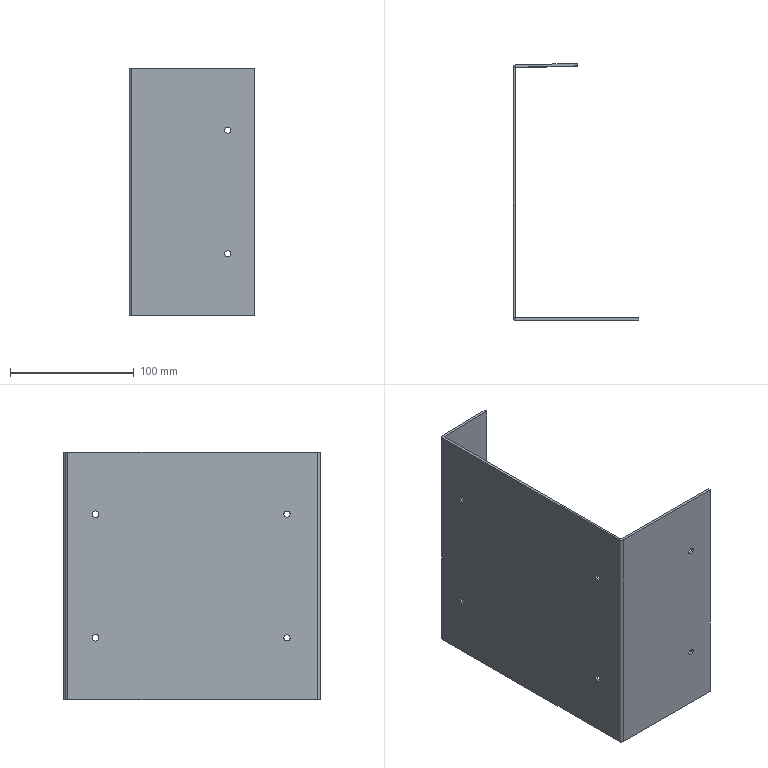Part | STEP file | TS-S55 | 1 solid | 34 faces | box 102 x 207.828 x 200 mm | volume 142020 mm3 | plane 18 | cylinder 16 | commonest cylinder face diameters 5 x8 5.4 x4 0.4 x2 4.4 x2